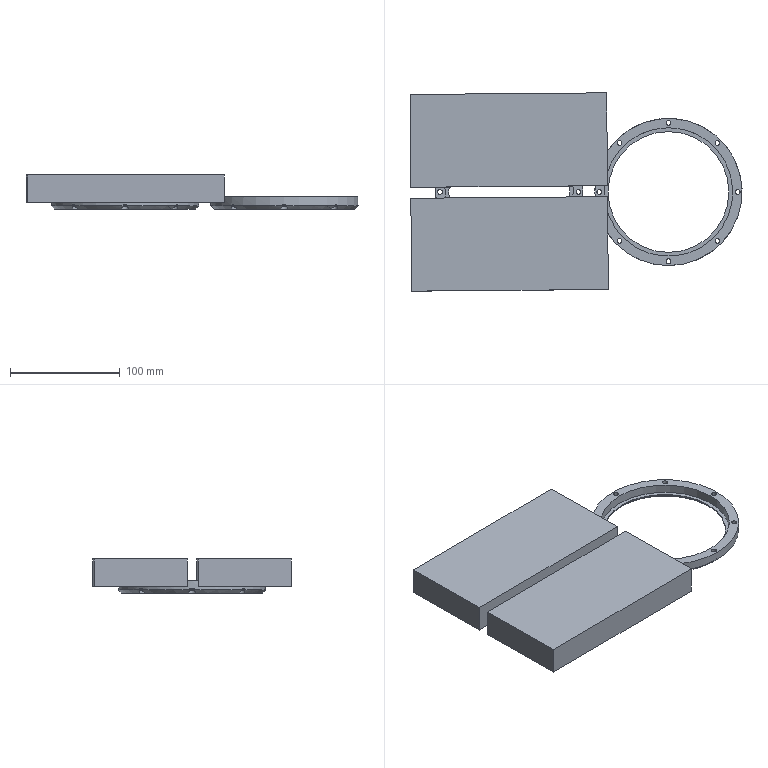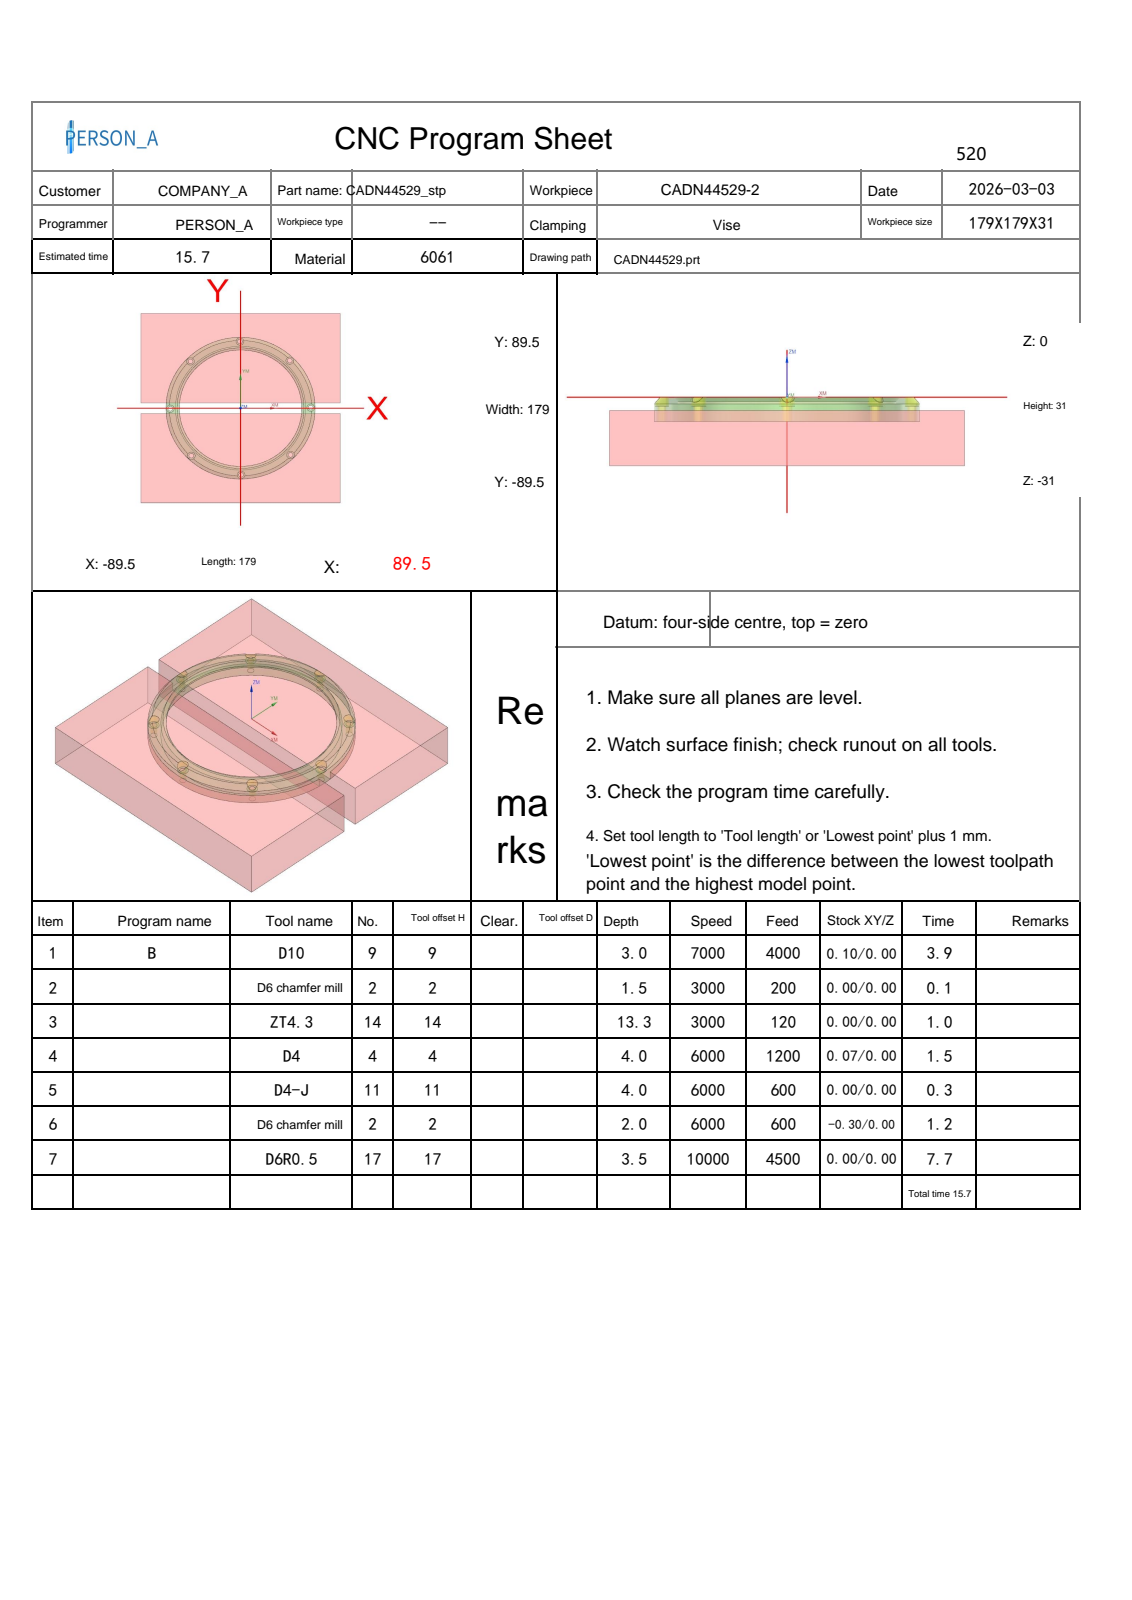NC program | NX | posted by the shop | part box 302.234 x 180.468 x 31 mm
Lines 1 to 1280 of 75694:
%
O0001
(Machine time: 16.93 MIN)
(===Total Tool:6===)
(T9=D10     D=10.  R=0.   D-  H09 Z=-3.   )
(T2=D6 chamfer mill   D=6.   R=0.   D-  H02 Z=-2.   )
(T14=ZT4.3  D=4.3  DR_a=118 D-  H14 Z=-13.29)
(T4=D4      D=4.   R=0.   D-  H04 Z=-4.   )
(T11=D4-J   D=4.   R=0.   D-  H11 Z=-4.   )
(T17=D6R0.5 D=6.   R=0.5  D-  H17 Z=-3.5  )
G80 G90 G17 G49 G40
G91 G28 Z0
M01
N1 T09 M06
(D10  D=10. R=0. H=09 ce=0.10 di=0.00)
G00 G90 G54 X42.81 Y-29.091 M03 S7000
G43 H09 Z50.
M08
Z1.5
G01 X42.978 Y-28.851 Z1.485 F4000.
X44.071 Y-27.151 Z1.379
X45.097 Y-25.411 Z1.273
X46.054 Y-23.632 Z1.167
X46.942 Y-21.816 Z1.061
X47.757 Y-19.968 Z.955
X48.5 Y-18.089 Z.849
X49.169 Y-16.182 Z.743
X49.763 Y-14.251 Z.637
X50.281 Y-12.298 Z.532
X50.723 Y-10.326 Z.426
X51.087 Y-8.339 Z.32
X51.374 Y-6.339 Z.214
X51.582 Y-4.329 Z.108
X51.712 Y-2.313 Z.002
X51.763 Y-.293 Z-.104
X51.757 Y.426 Z-.142
G03 X0.0 Y51.759 I-51.757 J-.426
X-51.759 Y0.0 I0.0 J-51.759
X0.0 Y-51.759 I51.759 J0.0
X51.759 Y0.0 I0.0 J51.759
X51.757 Y.426 I-51.759 J0.0
G01 X51.746 Y1.114
X51.727 Y1.801
X51.698 Y2.488
X51.66 Y3.175 Z-.143
X51.613 Y3.861
X51.557 Y4.547
X51.491 Y5.231 Z-.144
X51.417 Y5.915
X51.334 Y6.597
X51.241 Y7.279 Z-.145
X51.14 Y7.959
X51.029 Y8.638
X50.91 Y9.315
X50.781 Y9.99 Z-.146
X50.643 Y10.664
X50.497 Y11.336
X50.342 Y12.006 Z-.147
X50.177 Y12.673
X50.004 Y13.339
X49.822 Y14.002 Z-.148
X49.632 Y14.663
X49.432 Y15.321
X49.224 Y15.976
X49.007 Y16.629 Z-.149
X48.782 Y17.278
X48.547 Y17.925
X48.305 Y18.568 Z-.15
X48.053 Y19.208
X47.794 Y19.845
X47.526 Y20.478 Z-.151
X47.249 Y21.107
X46.964 Y21.733
X46.671 Y22.355
X46.37 Y22.973 Z-.152
X46.06 Y23.587
X45.742 Y24.197
X45.416 Y24.802 Z-.153
X45.083 Y25.403
X44.741 Y26.
X44.391 Y26.592
X44.109 Y27.057 Z-.154
X43.822 Y27.519
X43.746 Y27.64
X43.669 Y27.762
X43.278 Y28.365
X42.88 Y28.964 Z-.155
X42.473 Y29.556
X42.058 Y30.143
X41.635 Y30.724 Z-.156
X41.204 Y31.3
X40.765 Y31.869
X40.318 Y32.432 Z-.157
X39.864 Y32.989
X39.401 Y33.539
X38.931 Y34.083 Z-.158
X38.454 Y34.62
X37.969 Y35.151
X37.477 Y35.675
X36.978 Y36.192 Z-.159
X36.471 Y36.701
X35.957 Y37.204
X35.437 Y37.7 Z-.16
X34.91 Y38.188
X34.376 Y38.669
X33.835 Y39.143 Z-.161
X33.288 Y39.609
X32.734 Y40.067
X32.174 Y40.518 Z-.162
X31.608 Y40.961
X31.036 Y41.396
X30.457 Y41.822 Z-.163
X29.873 Y42.241
X29.284 Y42.652
X28.688 Y43.054
X28.087 Y43.448 Z-.164
X27.481 Y43.834
X26.869 Y44.211
X26.252 Y44.58 Z-.165
X25.63 Y44.94
X25.003 Y45.292
X24.371 Y45.634 Z-.166
X23.735 Y45.968
X23.094 Y46.293
X22.449 Y46.609 Z-.167
X21.799 Y46.916
X21.145 Y47.214
X20.487 Y47.503 Z-.168
X19.825 Y47.783
X19.159 Y48.053
X18.49 Y48.315
X17.817 Y48.566 Z-.169
X17.14 Y48.809
X16.46 Y49.042
X15.777 Y49.266 Z-.17
X15.091 Y49.48
X14.403 Y49.684
X13.711 Y49.879 Z-.171
X13.017 Y50.065
X12.32 Y50.24
X11.621 Y50.406 Z-.172
X10.919 Y50.563
X10.216 Y50.709
X9.51 Y50.846 Z-.173
X8.803 Y50.973
X8.094 Y51.09
X7.384 Y51.197
X6.672 Y51.294 Z-.174
X5.958 Y51.382
X5.244 Y51.459
X4.529 Y51.527 Z-.175
X3.812 Y51.584
X3.095 Y51.632
X2.378 Y51.67 Z-.176
X1.66 Y51.697
X.942 Y51.715
X.223 Y51.723 Z-.177
X-.495 Y51.721
X-1.214 Y51.709
X-1.932 Y51.686 Z-.178
X-2.65 Y51.654
X-3.367 Y51.612
X-4.084 Y51.56 Z-.179
X-4.799 Y51.498
X-5.514 Y51.426
X-6.228 Y51.344
X-6.941 Y51.253 Z-.18
X-7.652 Y51.151
X-8.362 Y51.039
X-9.07 Y50.918 Z-.181
X-9.776 Y50.787
X-10.481 Y50.646
X-11.183 Y50.495 Z-.182
X-11.883 Y50.334
X-12.581 Y50.164
X-13.277 Y49.984 Z-.183
X-13.97 Y49.795
X-14.66 Y49.596
X-15.348 Y49.387 Z-.184
X-16.032 Y49.169
X-16.713 Y48.941
X-17.392 Y48.704
X-18.066 Y48.457 Z-.185
X-18.738 Y48.201
X-19.405 Y47.936
X-20.069 Y47.661 Z-.186
X-20.729 Y47.378
X-21.385 Y47.085
X-22.037 Y46.783 Z-.187
X-22.685 Y46.472
X-23.328 Y46.152
X-23.967 Y45.823 Z-.188
X-24.601 Y45.486
X-25.23 Y45.139
X-25.854 Y44.784 Z-.189
X-26.474 Y44.421
X-27.088 Y44.048
X-27.697 Y43.667
X-28.301 Y43.278 Z-.19
X-28.899 Y42.881
X-29.492 Y42.475
X-30.079 Y42.061 Z-.191
X-30.66 Y41.639
X-31.236 Y41.208
X-31.805 Y40.77 Z-.192
X-32.368 Y40.324
X-32.925 Y39.871
X-33.475 Y39.409 Z-.193
X-34.019 Y38.94
X-34.557 Y38.464
X-35.087 Y37.98 Z-.194
X-35.611 Y37.488
X-36.128 Y36.99
X-36.639 Y36.484
X-37.142 Y35.971 Z-.195
X-37.637 Y35.452
X-38.126 Y34.925
X-38.607 Y34.392 Z-.196
X-39.081 Y33.852
X-39.547 Y33.306
X-40.006 Y32.753 Z-.197
X-40.457 Y32.194
X-40.9 Y31.629
X-41.335 Y31.057 Z-.198
X-41.762 Y30.48
X-42.181 Y29.897
X-42.592 Y29.308 Z-.199
X-42.995 Y28.713
X-43.39 Y28.113
X-43.715 Y27.603
X-44.035 Y27.09 Z-.2
X-44.094 Y26.993
X-44.153 Y26.896
X-44.521 Y26.282
X-44.881 Y25.663
X-45.231 Y25.039 Z-.201
X-45.574 Y24.41
X-45.907 Y23.776
X-46.232 Y23.138 Z-.202
X-46.547 Y22.495
X-46.854 Y21.848
X-47.152 Y21.197 Z-.203
X-47.441 Y20.542
X-47.72 Y19.883
X-47.991 Y19.22 Z-.204
X-48.252 Y18.553
X-48.504 Y17.883
X-48.747 Y17.21
X-48.98 Y16.533 Z-.205
X-49.204 Y15.853
X-49.419 Y15.17
X-49.624 Y14.484 Z-.206
X-49.819 Y13.795
X-50.005 Y13.104
X-50.182 Y12.41 Z-.207
X-50.349 Y11.714
X-50.506 Y11.015
X-50.653 Y10.315 Z-.208
X-50.791 Y9.612
X-50.919 Y8.908
X-51.037 Y8.202 Z-.209
X-51.145 Y7.494
X-51.244 Y6.785
X-51.332 Y6.074
X-51.411 Y5.363 Z-.21
X-51.48 Y4.65
X-51.54 Y3.937
X-51.589 Y3.223 Z-.211
X-51.628 Y2.508
X-51.658 Y1.793
X-51.677 Y1.077 Z-.212
X-51.687 Y.361
Y-.355
X-51.676 Y-1.07 Z-.213
X-51.656 Y-1.786
X-51.626 Y-2.501
X-51.586 Y-3.216
X-51.537 Y-3.93 Z-.214
X-51.477 Y-4.643
X-51.407 Y-5.356
X-51.328 Y-6.067 Z-.215
X-51.239 Y-6.777
X-51.14 Y-7.486
X-51.031 Y-8.194 Z-.216
X-50.912 Y-8.9
X-50.784 Y-9.604
X-50.645 Y-10.306 Z-.217
X-50.498 Y-11.006
X-50.34 Y-11.705
X-50.173 Y-12.401 Z-.218
X-49.996 Y-13.094
X-49.81 Y-13.785
X-49.614 Y-14.474
X-49.408 Y-15.159 Z-.219
X-49.193 Y-15.842
X-48.969 Y-16.522
X-48.735 Y-17.198 Z-.22
X-48.492 Y-17.871
X-48.239 Y-18.541
X-47.978 Y-19.207 Z-.221
X-47.707 Y-19.87
X-47.427 Y-20.529
X-47.137 Y-21.183 Z-.222
X-46.839 Y-21.834
X-46.532 Y-22.48
X-46.216 Y-23.122 Z-.223
X-45.891 Y-23.76
X-45.557 Y-24.393
X-45.215 Y-25.022
X-44.864 Y-25.645 Z-.224
X-44.504 Y-26.264
X-44.136 Y-26.878
X-43.759 Y-27.486 Z-.225
X-43.374 Y-28.09
X-42.98 Y-28.687
X-42.579 Y-29.28 Z-.226
X-42.169 Y-29.866
X-41.751 Y-30.447
X-41.325 Y-31.022 Z-.227
X-40.891 Y-31.592
X-40.45 Y-32.155
X-40. Y-32.712 Z-.228
X-39.543 Y-33.262
X-39.078 Y-33.806
X-38.606 Y-34.344
X-38.127 Y-34.875 Z-.229
X-37.64 Y-35.4
X-37.146 Y-35.918
X-36.644 Y-36.428 Z-.23
X-36.136 Y-36.932
X-35.621 Y-37.429
X-35.099 Y-37.918 Z-.231
X-34.57 Y-38.4
X-34.035 Y-38.875
X-33.493 Y-39.343 Z-.232
X-32.945 Y-39.803
X-32.39 Y-40.255
X-31.829 Y-40.699 Z-.233
X-31.263 Y-41.136
X-30.69 Y-41.565
X-30.111 Y-41.985
X-29.526 Y-42.398 Z-.234
X-28.936 Y-42.803
X-28.34 Y-43.199
X-27.739 Y-43.587 Z-.235
X-27.133 Y-43.967
X-26.521 Y-44.338
X-25.904 Y-44.701 Z-.236
X-25.283 Y-45.055
X-24.656 Y-45.401
X-24.025 Y-45.738 Z-.237
X-23.389 Y-46.066
X-22.749 Y-46.385
X-22.104 Y-46.695
X-21.455 Y-46.997 Z-.238
X-20.802 Y-47.289
X-20.145 Y-47.572
X-19.484 Y-47.846 Z-.239
X-18.819 Y-48.111
X-18.151 Y-48.367
X-17.479 Y-48.613 Z-.24
X-16.804 Y-48.851
X-16.126 Y-49.078
X-15.445 Y-49.297 Z-.241
X-14.761 Y-49.506
X-14.073 Y-49.705
X-13.384 Y-49.895 Z-.242
X-12.691 Y-50.075
X-11.996 Y-50.246
X-11.299 Y-50.407
X-10.6 Y-50.558 Z-.243
X-9.899 Y-50.7
X-9.196 Y-50.832
X-8.491 Y-50.954 Z-.244
X-7.784 Y-51.066
X-7.076 Y-51.169
X-6.367 Y-51.262 Z-.245
X-5.787 Y-51.33
X-5.207 Y-51.392
X-5.13 Y-51.4
X-5.052 Y-51.407
X-4.393 Y-51.467 Z-.246
X-3.734 Y-51.519
X-3.074 Y-51.562
X-2.414 Y-51.597
X-1.753 Y-51.624 Z-.247
X-1.092 Y-51.642
X-.43 Y-51.651
X.231 Y-51.652 Z-.248
X.893 Y-51.645
X1.554 Y-51.629
X2.215 Y-51.604
X2.875 Y-51.571 Z-.249
X3.535 Y-51.53
X4.195 Y-51.48
X4.701 Y-51.436
X5.207 Y-51.387 Z-.25
X5.359 Y-51.372
X5.512 Y-51.355
X6.224 Y-51.274
X6.936 Y-51.182
X7.646 Y-51.08 Z-.251
X8.354 Y-50.969
X9.061 Y-50.848
X9.767 Y-50.717 Z-.252
X10.47 Y-50.576
X11.171 Y-50.425
X11.87 Y-50.265 Z-.253
X12.567 Y-50.095
X13.261 Y-49.915
X13.953 Y-49.726 Z-.254
X14.642 Y-49.527
X15.329 Y-49.319
X16.012 Y-49.101 Z-.255
X16.692 Y-48.873
X17.369 Y-48.636
X18.043 Y-48.39
X18.713 Y-48.135 Z-.256
X19.38 Y-47.87
X20.043 Y-47.596
X20.701 Y-47.313 Z-.257
X21.356 Y-47.02
X22.007 Y-46.719
X22.654 Y-46.409 Z-.258
X23.296 Y-46.089
X23.934 Y-45.761
X24.567 Y-45.424 Z-.259
X25.195 Y-45.078
X25.818 Y-44.724
X26.437 Y-44.36 Z-.26
X27.05 Y-43.989
X27.658 Y-43.609
X28.261 Y-43.22
X28.858 Y-42.823 Z-.261
X29.45 Y-42.418
X30.036 Y-42.005
X30.616 Y-41.583 Z-.262
X31.191 Y-41.154
X31.759 Y-40.716
X32.321 Y-40.271 Z-.263
X32.877 Y-39.818
X33.427 Y-39.357
X33.97 Y-38.889 Z-.264
X34.507 Y-38.413
X35.036 Y-37.93
X35.56 Y-37.44 Z-.265
X36.076 Y-36.942
X36.585 Y-36.437
X37.088 Y-35.926
X37.583 Y-35.407 Z-.266
X38.071 Y-34.881
X38.551 Y-34.349
X39.024 Y-33.81 Z-.267
X39.49 Y-33.265
X39.948 Y-32.713
X40.398 Y-32.155 Z-.268
X40.84 Y-31.591
X41.275 Y-31.02
X41.701 Y-30.444 Z-.269
X42.12 Y-29.862
X42.53 Y-29.274
X42.932 Y-28.68 Z-.27
X43.326 Y-28.081
X43.712 Y-27.476
X44.089 Y-26.866
X44.457 Y-26.251 Z-.271
X44.817 Y-25.631
X45.169 Y-25.006
X45.511 Y-24.376 Z-.272
X45.845 Y-23.742
X46.17 Y-23.103
X46.486 Y-22.459 Z-.273
X46.794 Y-21.811
X47.092 Y-21.159
X47.381 Y-20.503 Z-.274
X47.661 Y-19.843
X47.931 Y-19.179
X48.193 Y-18.511 Z-.275
X48.445 Y-17.84
X48.688 Y-17.166
X48.921 Y-16.488
X49.145 Y-15.807 Z-.276
X49.359 Y-15.123
X49.564 Y-14.436
X49.76 Y-13.746 Z-.277
X49.946 Y-13.053
X50.122 Y-12.358
X50.288 Y-11.661 Z-.278
X50.445 Y-10.961
X50.592 Y-10.26
X50.729 Y-9.556 Z-.279
X50.857 Y-8.851
X50.975 Y-8.143
X51.082 Y-7.435 Z-.28
X51.18 Y-6.725
X51.269 Y-6.013
X51.347 Y-5.301
X51.415 Y-4.587 Z-.281
X51.474 Y-3.872
X51.522 Y-3.157
X51.561 Y-2.441 Z-.282
X51.589 Y-1.725
X51.608 Y-1.008
X51.617 Y-.292 Z-.283
X51.615 Y.425
X51.604 Y1.138
X51.583 Y1.851 Z-.284
X51.553 Y2.563
X51.512 Y3.275
X51.461 Y3.986
X51.401 Y4.696 Z-.285
X51.331 Y5.406
X51.251 Y6.114
X51.162 Y6.821 Z-.286
X51.062 Y7.527
X50.953 Y8.232
X50.834 Y8.935 Z-.287
X50.706 Y9.636
X50.567 Y10.335
X50.42 Y11.033 Z-.288
X50.262 Y11.728
X50.095 Y12.421
X49.918 Y13.111 Z-.289
X49.732 Y13.8
X49.537 Y14.485
X49.331 Y15.168
X49.117 Y15.848 Z-.29
X48.893 Y16.524
X48.66 Y17.198
X48.417 Y17.868 Z-.291
X48.166 Y18.535
X47.905 Y19.199
X47.635 Y19.858 Z-.292
X47.356 Y20.514
X47.068 Y21.166
X46.771 Y21.814 Z-.293
X46.464 Y22.458
X46.15 Y23.097
X45.826 Y23.732 Z-.294
X45.493 Y24.363
X45.152 Y24.989
X44.803 Y25.61
X44.444 Y26.226 Z-.295
X44.078 Y26.837
X43.703 Y27.443
X43.679 Y27.48
X43.656 Y27.517
X43.293 Y28.085 Z-.296
X42.922 Y28.647
X42.52 Y29.241
X42.109 Y29.829 Z-.297
X41.69 Y30.411
X41.263 Y30.987
X40.828 Y31.558 Z-.298
X40.385 Y32.122
X39.935 Y32.68
X39.476 Y33.232 Z-.299
X39.01 Y33.777
X38.537 Y34.316
X38.056 Y34.848
X37.568 Y35.373 Z-.3
X37.072 Y35.892
X36.57 Y36.403
X36.06 Y36.908 Z-.301
X35.543 Y37.405
X35.02 Y37.895
X34.489 Y38.378 Z-.302
X33.952 Y38.854
X33.409 Y39.322
X32.859 Y39.782 Z-.303
X32.303 Y40.234
X31.74 Y40.679
X31.171 Y41.116 Z-.304
X30.597 Y41.545
X30.016 Y41.966
X29.43 Y42.379
X28.838 Y42.784 Z-.305
X28.24 Y43.18
X27.637 Y43.568
X27.029 Y43.948 Z-.306
X26.415 Y44.319
X25.796 Y44.682
X25.173 Y45.036 Z-.307
X24.544 Y45.381
X23.911 Y45.718
X23.273 Y46.045 Z-.308
X22.63 Y46.364
X21.984 Y46.674
X21.333 Y46.974 Z-.309
X20.678 Y47.266
X20.019 Y47.549
X19.356 Y47.822
X18.689 Y48.086 Z-.31
X18.019 Y48.341
X17.345 Y48.587
X16.668 Y48.823 Z-.311
X15.988 Y49.049
X15.304 Y49.266
X14.618 Y49.474 Z-.312
X13.929 Y49.672
X13.237 Y49.861
X12.542 Y50.04 Z-.313
X11.846 Y50.209
X11.147 Y50.368
X10.445 Y50.518 Z-.314
X9.742 Y50.658
X9.037 Y50.788
X8.33 Y50.909
X7.622 Y51.019 Z-.315
X6.912 Y51.12
X6.201 Y51.211
X5.488 Y51.292 Z-.316
X4.775 Y51.363
X4.06 Y51.424
X3.345 Y51.475 Z-.317
X2.629 Y51.516
X1.913 Y51.547
X1.196 Y51.569 Z-.318
X.48 Y51.58
X-.237 Y51.581
X-.954 Y51.573 Z-.319
X-1.671 Y51.554
X-2.387 Y51.526
X-3.103 Y51.487 Z-.32
X-3.819 Y51.439
X-4.533 Y51.38
X-5.247 Y51.312
X-5.96 Y51.234 Z-.321
X-6.671 Y51.146
X-7.381 Y51.048
X-8.09 Y50.94 Z-.322
X-8.797 Y50.822
X-9.503 Y50.695
X-10.206 Y50.558 Z-.323
X-10.908 Y50.411
X-11.608 Y50.254
X-12.305 Y50.087 Z-.324
X-13. Y49.911
X-13.692 Y49.725
X-14.382 Y49.53 Z-.325
X-15.069 Y49.325
X-15.753 Y49.11
X-16.434 Y48.886
X-17.112 Y48.653 Z-.326
X-17.786 Y48.41
X-18.457 Y48.158
X-19.125 Y47.896 Z-.327
X-19.788 Y47.626
X-20.448 Y47.346
X-21.104 Y47.057 Z-.328
X-21.756 Y46.759
X-22.404 Y46.451
X-23.047 Y46.135 Z-.329
X-23.686 Y45.81
X-24.32 Y45.476
X-24.95 Y45.133 Z-.33
X-25.575 Y44.782
X-26.194 Y44.422
X-26.809 Y44.053
X-27.419 Y43.676 Z-.331
X-28.023 Y43.291
X-28.622 Y42.897
X-29.215 Y42.494 Z-.332
X-29.803 Y42.084
X-30.385 Y41.666
X-30.961 Y41.239 Z-.333
X-31.531 Y40.804
X-32.094 Y40.362
X-32.652 Y39.912 Z-.334
X-33.204 Y39.454
X-33.749 Y38.988
X-34.287 Y38.515 Z-.335
X-34.819 Y38.035
X-35.344 Y37.547
X-35.862 Y37.052
X-36.373 Y36.549 Z-.336
X-36.878 Y36.04
X-37.375 Y35.524
X-37.865 Y35.001 Z-.337
X-38.347 Y34.471
X-38.822 Y33.934
X-39.29 Y33.391 Z-.338
X-39.75 Y32.842
X-40.203 Y32.286
X-40.647 Y31.724 Z-.339
X-41.084 Y31.155
X-41.513 Y30.581
X-41.934 Y30.001 Z-.34
X-42.346 Y29.415
X-42.751 Y28.824
X-43.147 Y28.226
X-43.535 Y27.624 Z-.341
X-43.914 Y27.016
X-43.935 Y26.983
X-43.955 Y26.95
X-44.304 Y26.372
X-44.645 Y25.789 Z-.342
X-44.997 Y25.169
X-45.341 Y24.543
X-45.676 Y23.913 Z-.343
X-46.003 Y23.278
X-46.32 Y22.639
X-46.629 Y21.995 Z-.344
X-46.929 Y21.348
X-47.22 Y20.696
X-47.501 Y20.04 Z-.345
X-47.774 Y19.38
X-48.037 Y18.717
X-48.292 Y18.05
X-48.537 Y17.38 Z-.346
X-48.772 Y16.706
X-48.999 Y16.029
X-49.215 Y15.349 Z-.347
X-49.423 Y14.666
X-49.621 Y13.98
X-49.809 Y13.292 Z-.348
X-49.988 Y12.601
X-50.158 Y11.908
X-50.317 Y11.212 Z-.349
X-50.468 Y10.514
X-50.608 Y9.814
X-50.739 Y9.113 Z-.35
X-50.86 Y8.41
X-50.971 Y7.705
X-51.072 Y6.998
X-51.164 Y6.29 Z-.351
X-51.246 Y5.581
X-51.318 Y4.871
X-51.38 Y4.16 Z-.352
X-51.433 Y3.449
X-51.475 Y2.736
X-51.508 Y2.023 Z-.353
X-51.531 Y1.31
X-51.543 Y.596
X-51.546 Y-.117 Z-.354
X-51.54 Y-.831
X-51.523 Y-1.544
X-51.496 Y-2.257
X-51.46 Y-2.97 Z-.355
X-51.413 Y-3.682
X-51.357 Y-4.394
X-51.291 Y-5.104 Z-.356
X-51.215 Y-5.814
X-51.129 Y-6.522
X-51.034 Y-7.229 Z-.357
X-50.929 Y-7.935
X-50.814 Y-8.639
X-50.689 Y-9.342 Z-.358
X-50.554 Y-10.043
X-50.41 Y-10.742
X-50.256 Y-11.438 Z-.359
X-50.093 Y-12.133
X-49.92 Y-12.825
X-49.737 Y-13.515
X-49.545 Y-14.202 Z-.36
X-49.343 Y-14.887
X-49.132 Y-15.568
X-48.912 Y-16.247 Z-.361
X-48.682 Y-16.922
X-48.442 Y-17.595
X-48.194 Y-18.263 Z-.362
X-47.936 Y-18.929
X-47.669 Y-19.591
X-47.393 Y-20.249 Z-.363
X-47.108 Y-20.903
X-46.814 Y-21.553
X-46.511 Y-22.199 Z-.364
X-46.199 Y-22.84
X-45.878 Y-23.477
X-45.548 Y-24.11
X-45.21 Y-24.738 Z-.365
X-44.862 Y-25.362
X-44.507 Y-25.98
X-44.143 Y-26.594 Z-.366
X-43.77 Y-27.202
X-43.389 Y-27.805
X-43. Y-28.403 Z-.367
X-42.602 Y-28.996
X-42.196 Y-29.582
X-41.782 Y-30.164 Z-.368
X-41.36 Y-30.739
X-40.931 Y-31.308
X-40.493 Y-31.872 Z-.369
X-40.048 Y-32.429
X-39.595 Y-32.98
X-39.134 Y-33.525
X-38.666 Y-34.063 Z-.37
X-38.19 Y-34.595
X-37.708 Y-35.12
X-37.218 Y-35.639 Z-.371
X-36.72 Y-36.151
X-36.216 Y-36.655
X-35.705 Y-37.153 Z-.372
X-35.187 Y-37.643
X-34.662 Y-38.127
X-34.131 Y-38.603 Z-.373
X-33.593 Y-39.071
X-33.049 Y-39.532
X-32.498 Y-39.986 Z-.374
X-31.941 Y-40.432
X-31.378 Y-40.87
X-30.809 Y-41.3
X-30.234 Y-41.722 Z-.375
X-29.653 Y-42.137
X-29.067 Y-42.543
X-28.475 Y-42.941 Z-.376
X-27.878 Y-43.331
X-27.275 Y-43.712
X-26.667 Y-44.086 Z-.377
X-26.054 Y-44.45
X-25.436 Y-44.806
X-24.813 Y-45.154 Z-.378
X-24.185 Y-45.493
X-23.553 Y-45.823
X-22.916 Y-46.144
X-22.275 Y-46.457 Z-.379
X-21.63 Y-46.761
X-20.98 Y-47.055
X-20.327 Y-47.341 Z-.38
X-19.669 Y-47.618
X-19.008 Y-47.885
X-18.343 Y-48.143 Z-.381
X-17.675 Y-48.392
X-17.003 Y-48.632
X-16.328 Y-48.863 Z-.382
X-15.65 Y-49.084
X-14.969 Y-49.295
X-14.285 Y-49.498 Z-.383
X-13.598 Y-49.69
X-12.909 Y-49.873
X-12.217 Y-50.047
X-11.523 Y-50.211 Z-.384
X-10.827 Y-50.366
X-10.128 Y-50.51
X-9.428 Y-50.645 Z-.385
X-8.726 Y-50.771
X-8.022 Y-50.886
X-7.328 Y-50.991 Z-.386
X-6.61 Y-51.088
X-5.902 Y-51.175
X-5.193 Y-51.251 Z-.387
X-4.546 Y-51.312
X-3.898 Y-51.365
X-3.249 Y-51.41
X-2.6 Y-51.447 Z-.388
X-1.95 Y-51.475
X-1.3 Y-51.495
X-.65 Y-51.507 Z-.389
X0.0 Y-51.511
X.65 Y-51.507
X1.3 Y-51.494
X1.95 Y-51.473 Z-.39
X2.6 Y-51.444
X3.249 Y-51.407
X3.897 Y-51.362 Z-.391
X4.545 Y-51.308
X5.193 Y-51.247
X5.359 Y-51.229
X5.524 Y-51.212
X6.059 Y-51.151 Z-.392
X6.593 Y-51.085
X7.292 Y-50.989
X7.989 Y-50.884
X8.684 Y-50.77 Z-.393
X9.378 Y-50.646
X10.07 Y-50.513
X10.761 Y-50.37 Z-.394
X11.449 Y-50.218
X12.135 Y-50.056
X12.819 Y-49.885 Z-.395
X13.5 Y-49.705
X14.179 Y-49.515
X14.855 Y-49.316
X15.529 Y-49.108 Z-.396
X16.199 Y-48.89
X16.867 Y-48.664
X17.531 Y-48.428 Z-.397
X18.192 Y-48.183
X18.85 Y-47.929
X19.504 Y-47.667 Z-.398
X20.154 Y-47.395
X20.801 Y-47.115
X21.443 Y-46.825 Z-.399
X22.082 Y-46.527
X22.716 Y-46.22
X23.347 Y-45.905
X23.973 Y-45.581 Z-.4
X24.594 Y-45.248
X25.211 Y-44.907
X25.823 Y-44.558 Z-.401
X26.43 Y-44.2
X27.032 Y-43.834
X27.629 Y-43.459 Z-.402
X28.221 Y-43.077
X28.808 Y-42.686
X29.389 Y-42.288 Z-.403
X29.965 Y-41.881
X30.535 Y-41.467
X31.1 Y-41.045
X31.658 Y-40.615 Z-.404
X32.211 Y-40.178
X32.758 Y-39.733
X33.298 Y-39.281 Z-.405
X33.832 Y-38.822
X34.36 Y-38.355
X34.882 Y-37.881 Z-.406
X35.397 Y-37.399
X35.905 Y-36.911
X36.407 Y-36.416 Z-.407
X36.901 Y-35.914
X37.389 Y-35.406
X37.87 Y-34.891
X38.344 Y-34.369 Z-.408
X38.81 Y-33.841
X39.269 Y-33.306
X39.721 Y-32.766 Z-.409
X40.166 Y-32.219
X40.603 Y-31.666
X41.032 Y-31.107 Z-.41
X41.454 Y-30.542
X41.868 Y-29.972
X42.274 Y-29.396 Z-.411
X42.672 Y-28.815
X43.062 Y-28.228
X43.444 Y-27.636
X43.818 Y-27.038 Z-.412
X44.183 Y-26.436
X44.541 Y-25.829
X44.89 Y-25.217 Z-.413
X45.23 Y-24.6
X45.562 Y-23.978
X45.886 Y-23.352 Z-.414
X46.201 Y-22.722
X46.507 Y-22.088
X46.805 Y-21.449 Z-.415
X47.094 Y-20.806
X47.374 Y-20.16
X47.645 Y-19.509
X47.907 Y-18.855 Z-.416
X48.161 Y-18.198
X48.405 Y-17.537
X48.64 Y-16.873 Z-.417
X48.866 Y-16.206
X49.083 Y-15.535
X49.291 Y-14.862 Z-.418
X49.489 Y-14.186
X49.678 Y-13.507
X49.858 Y-12.826 Z-.419
X50.029 Y-12.142
X50.19 Y-11.457
X50.342 Y-10.769
X50.484 Y-10.079 Z-.42
X50.617 Y-9.387
X50.74 Y-8.693
X50.854 Y-7.998 Z-.421
X50.959 Y-7.301
X51.054 Y-6.603
X51.139 Y-5.904 Z-.422
X51.215 Y-5.203
X51.281 Y-4.502
X51.337 Y-3.8 Z-.423
X51.384 Y-3.097
X51.421 Y-2.393
X51.449 Y-1.689
X51.467 Y-.985 Z-.424
X51.475 Y-.28
X51.474 Y.424
X51.463 Y1.137 Z-.425
X51.442 Y1.85
X51.411 Y2.562
X51.37 Y3.274 Z-.426
X51.32 Y3.986
X51.259 Y4.696
X51.189 Y5.406 Z-.427
X51.109 Y6.115
X51.019 Y6.822
X50.919 Y7.528
X50.81 Y8.233 Z-.428
X50.69 Y8.936
X50.561 Y9.637
X50.423 Y10.337 Z-.429
X50.274 Y11.034
X50.116 Y11.73
X49.949 Y12.423 Z-.43
X49.772 Y13.113
X49.585 Y13.802
X49.389 Y14.487 Z-.431
X49.183 Y15.17
X48.968 Y15.85
X48.743 Y16.527 Z-.432
X48.509 Y17.2
X48.266 Y17.87
X48.013 Y18.537
X47.752 Y19.201 Z-.433
X47.481 Y19.86
X47.201 Y20.516
X46.912 Y21.168 Z-.434
X46.614 Y21.816
X46.307 Y22.459
X45.991 Y23.098 Z-.435
X45.666 Y23.733
X45.333 Y24.363
X44.991 Y24.989 Z-.436
X44.64 Y25.61
X44.28 Y26.226
X43.913 Y26.836 Z-.437
X43.536 Y27.442
X43.513 Y27.479
X43.489 Y27.516
X43.126 Y28.081
X42.756 Y28.641
X42.354 Y29.232 Z-.438
X41.943 Y29.818
X41.524 Y30.398
X41.098 Y30.972 Z-.439
X40.663 Y31.54
X40.221 Y32.102
X39.77 Y32.657 Z-.44
X39.312 Y33.207
X38.847 Y33.75
X38.374 Y34.286 Z-.441
X37.893 Y34.816
X37.406 Y35.339
X36.911 Y35.855 Z-.442
X36.409 Y36.364
X35.899 Y36.867
X35.383 Y37.362
X34.86 Y37.85 Z-.443
X34.331 Y38.33
X33.795 Y38.804
X33.252 Y39.269 Z-.444
X32.703 Y39.727
X32.147 Y40.178
X31.586 Y40.62 Z-.445
X31.018 Y41.055
X30.444 Y41.482
X29.864 Y41.901 Z-.446
X29.279 Y42.312
X28.688 Y42.714
X28.091 Y43.109 Z-.447
X27.489 Y43.495
X26.882 Y43.872
X26.27 Y44.241
X25.652 Y44.602 Z-.448
X25.029 Y44.954
X24.402 Y45.297
X23.77 Y45.631 Z-.449
X23.133 Y45.957
X22.492 Y46.274
X21.847 Y46.582 Z-.45
X21.197 Y46.881
X20.544 Y47.17
X19.886 Y47.451 Z-.451
X19.224 Y47.723
X18.559 Y47.985
X17.89 Y48.238 Z-.452
X17.218 Y48.481
X16.543 Y48.716
X15.864 Y48.941 Z-.453
X15.182 Y49.156
X14.497 Y49.362
X13.81 Y49.559
X13.12 Y49.745 Z-.454
X12.427 Y49.923
X11.732 Y50.09
X11.035 Y50.248 Z-.455
X10.335 Y50.396
X9.634 Y50.535
X8.93 Y50.663 Z-.456
X8.225 Y50.782
X7.519 Y50.891
X6.811 Y50.991 Z-.457
X6.101 Y51.08
X5.391 Y51.16
X4.679 Y51.229 Z-.458
X3.967 Y51.289
X3.253 Y51.339
X2.54 Y51.379
X1.825 Y51.409 Z-.459
X1.111 Y51.429
X.396 Y51.439
X-.319 Z-.46
X-1.034 Y51.43
X-1.749 Y51.41
X-2.463 Y51.38 Z-.461
X-3.177 Y51.341
X-3.89 Y51.292
X-4.602 Y51.232 Z-.462
X-5.314 Y51.163
X-6.025 Y51.084
X-6.734 Y50.995 Z-.463
X-7.442 Y50.896
X-8.148 Y50.787
X-8.853 Y50.669
X-9.557 Y50.541 Z-.464
X-10.258 Y50.403
X-10.958 Y50.255
X-11.655 Y50.098 Z-.465
X-12.35 Y49.93
X-13.043 Y49.754
X-13.733 Y49.567 Z-.466
X-14.42 Y49.371
X-15.105 Y49.166
X-15.787 Y48.951 Z-.467
X-16.465 Y48.726
X-17.141 Y48.493
X-17.813 Y48.249 Z-.468
X-18.482 Y47.997
X-19.147 Y47.735
X-19.808 Y47.464
X-20.466 Y47.184 Z-.469
X-21.12 Y46.895
X-21.769 Y46.596
X-22.415 Y46.289 Z-.47
X-23.056 Y45.973
X-23.692 Y45.648
X-24.324 Y45.314 Z-.471
X-24.951 Y44.971
X-25.574 Y44.62
X-26.191 Y44.26 Z-.472
X-26.804 Y43.891
X-27.411 Y43.514
X-28.013 Y43.129 Z-.473
X-28.609 Y42.735
X-29.2 Y42.333
X-29.786 Y41.923
X-30.365 Y41.504 Z-.474
X-30.939 Y41.078
X-31.507 Y40.644
X-32.068 Y40.202 Z-.475
X-32.624 Y39.752
X-33.173 Y39.295
X-33.716 Y38.829 Z-.476
X-34.252 Y38.357
X-34.781 Y37.877
X-35.304 Y37.39 Z-.477
X-35.82 Y36.895
X-36.329 Y36.394
X-36.831 Y35.885 Z-.478
X-37.326 Y35.369
X-37.814 Y34.847
X-38.294 Y34.318
X-38.767 Y33.782 Z-.479
X-39.233 Y33.24
X-39.691 Y32.691
X-40.141 Y32.136 Z-.48
X-40.584 Y31.575
X-41.018 Y31.008
X-41.445 Y30.435 Z-.481
X-41.864 Y29.855
X-42.274 Y29.271
X-42.677 Y28.68 Z-.482
X-43.071 Y28.084
X-43.457 Y27.482
X-43.834 Y26.876 Z-.483
X-43.894 Y26.779
X-43.953 Y26.681
X-44.26 Y26.169
X-44.561 Y25.653
X-44.911 Y25.034
X-45.252 Y24.41 Z-.484
X-45.585 Y23.782
X-45.91 Y23.149
X-46.225 Y22.511 Z-.485
X-46.532 Y21.87
X-46.83 Y21.224
X-47.118 Y20.574 Z-.486
X-47.398 Y19.92
X-47.669 Y19.263
X-47.93 Y18.602 Z-.487
X-48.183 Y17.937
X-48.426 Y17.269
X-48.66 Y16.597 Z-.488
X-48.885 Y15.922
X-49.1 Y15.245
X-49.306 Y14.564
X-49.502 Y13.881 Z-.489
X-49.689 Y13.195
X-49.866 Y12.506
X-50.034 Y11.815 Z-.49
X-50.193 Y11.122
X-50.341 Y10.427
X-50.48 Y9.729 Z-.491
X-50.61 Y9.03
X-50.73 Y8.329
X-50.84 Y7.627 Z-.492
X-50.94 Y6.923
X-51.031 Y6.218
X-51.111 Y5.511 Z-.493
X-51.182 Y4.804
X-51.244 Y4.095
X-51.295 Y3.386
X-51.337 Y2.676 Z-.494
X-51.368 Y1.966
X-51.39 Y1.255
X-51.403 Y.545 Z-.495
X-51.405 Y-.166
X-51.397 Y-.877
X-51.38 Y-1.588 Z-.496
X-51.353 Y-2.299
X-51.316 Y-3.009
X-51.269 Y-3.718 Z-.497
X-51.212 Y-4.427
X-51.146 Y-5.135
X-51.07 Y-5.841
X-50.984 Y-6.547 Z-.498
X-50.888 Y-7.252
X-50.782 Y-7.955
X-50.667 Y-8.656 Z-.499
X-50.542 Y-9.356
X-50.408 Y-10.054
X-50.264 Y-10.75 Z-.5
X-50.11 Y-11.444
X-49.946 Y-12.136
X-49.774 Y-12.826 Z-.501
X-49.591 Y-13.513
X-49.399 Y-14.198
X-49.198 Y-14.879 Z-.502
X-48.987 Y-15.558
X-48.767 Y-16.234
X-48.537 Y-16.907
X-48.299 Y-17.577 Z-.503
X-48.051 Y-18.243
X-47.793 Y-18.905
X-47.527 Y-19.565 Z-.504
X-47.252 Y-20.22
X-46.967 Y-20.871
X-46.674 Y-21.519 Z-.505
X-46.371 Y-22.162
X-46.06 Y-22.801
X-45.74 Y-23.436 Z-.506
X-45.411 Y-24.066
X-45.074 Y-24.692
X-44.728 Y-25.313 Z-.507
X-44.373 Y-25.929
X-44.01 Y-26.54
X-43.638 Y-27.146
X-43.258 Y-27.747 Z-.508
X-42.87 Y-28.342
X-42.474 Y-28.932
X-42.07 Y-29.517 Z-.509
X-41.657 Y-30.095
X-41.237 Y-30.669
X-40.808 Y-31.236 Z-.51
X-40.372 Y-31.797
X-39.928 Y-32.352
X-39.477 Y-32.901 Z-.511
X-39.018 Y-33.444
X-38.551 Y-33.98
X-38.077 Y-34.51 Z-.512
X-37.596 Y-35.033
X-37.108 Y-35.549
X-36.612 Y-36.059
X-36.11 Y-36.562 Z-.513
X-35.6 Y-37.057
X-35.084 Y-37.546
X-34.561 Y-38.027 Z-.514
X-34.032 Y-38.501
X-33.496 Y-38.968
X-32.954 Y-39.427 Z-.515
X-32.405 Y-39.879
X-31.85 Y-40.323
X-31.289 Y-40.76 Z-.516
X-30.722 Y-41.188
X-30.15 Y-41.609
X-29.571 Y-42.022
X-28.987 Y-42.427 Z-.517
X-28.397 Y-42.823
X-27.802 Y-43.212
X-27.201 Y-43.592 Z-.518
X-26.596 Y-43.963
X-25.985 Y-44.327
X-25.369 Y-44.682 Z-.519
X-24.749 Y-45.028
X-24.123 Y-45.366
X-23.494 Y-45.695 Z-.52
X-22.859 Y-46.015
X-22.22 Y-46.327